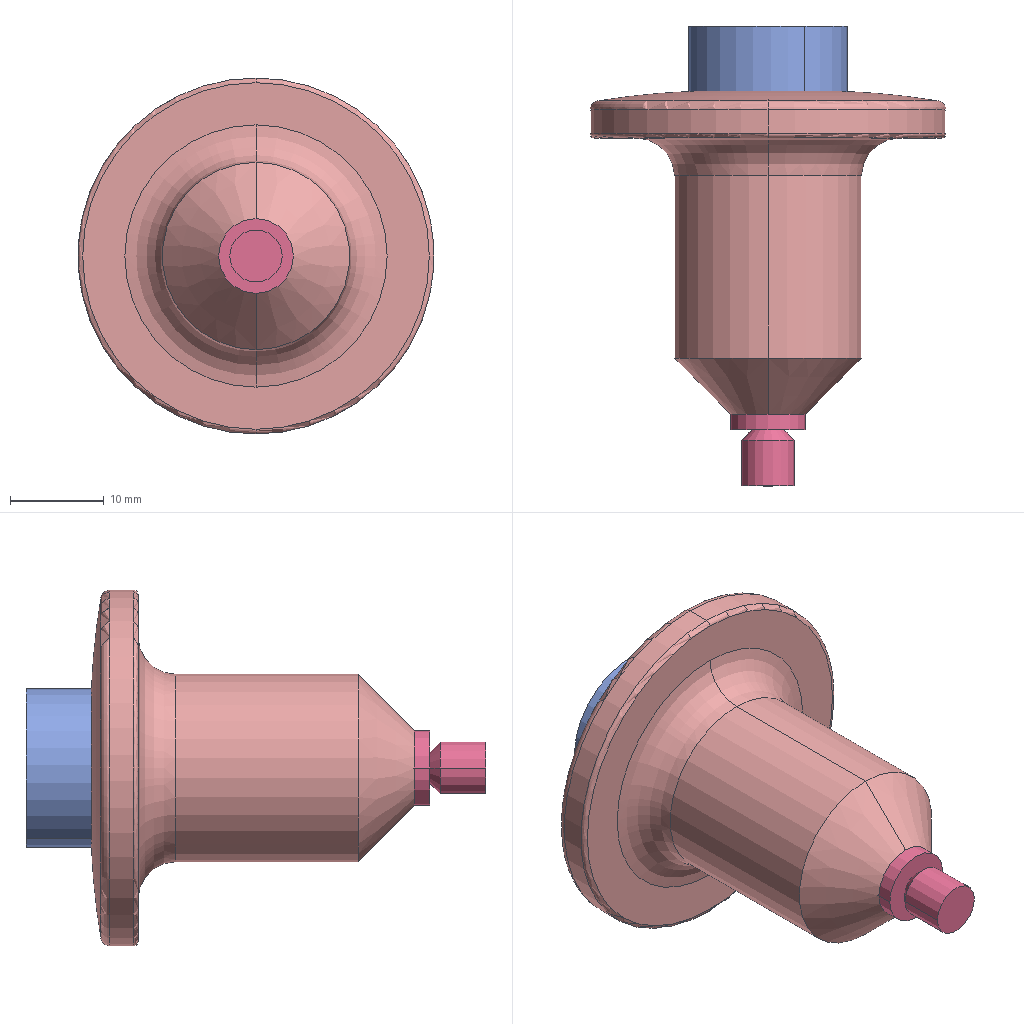Assembly | SolidWorks | 7 different items | 7 placed | box 38 x 49 x 38 mm
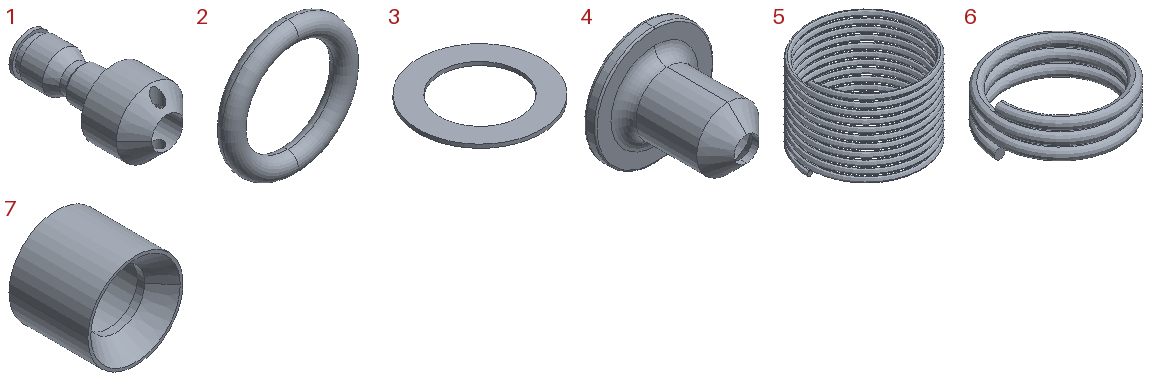Parts list (item | quantity | size | volume | features):
1 | x1 | 17 x 35.31 x 17 mm | 3384 mm3 | features Cut 1, ICE 1, MirrorPattern 1, RevCut 1, Revolution 1
2 | x1 | 12.043 x 1.84 x 12.043 mm | 85.235 mm3 | features Sweep 1
3 | x1 | 17 x 17 x 0.5 mm | 65.973 mm3 | features Extrusion 1
4 | x1 | 38 x 34.477 x 38 mm | 6932 mm3 | features Cut 1, ICE 1, Revolution 1
5 | x1 | 5.75 x 5.75 x 4.25 mm | 9.284 mm3 | features Helix 1, Sweep 1
6 | x1 | 17 x 17 x 6.999 mm | 258.247 mm3 | features Helix 1, Sweep 1
7 | x1 | 17 x 14.11 x 17 mm | 1515 mm3 | features Revolution 1
Mates (type | each side: item.copy, entity, surface, feature):
Concentric | 4.1 face cylinder Revolve1 | 7.1 face cylinder Revolve1
Concentric | 4.1 face cylinder Revolve1 | 1.1 face cylinder Revolve1
Concentric | 4.1 face cylinder Revolve1 | 6.1 select_type:24
Concentric | 1.1 edge | 5.1 select_type:24
Coincident | 1.1 face plane Cut-Extrude2 | 5.1 select_type:24
Concentric | 4.1 face cylinder Revolve1 | 3.1 face cylinder Boss-Extrude1
Coincident | 1.1 face plane Revolve1 | 6.1 select_type:24
Coincident | 4.1 edge | 3.1 face plane Boss-Extrude1
Concentric | 1.1 face cylinder Revolve1 | 2.1 select_type:24
Coincident | 1.1 face plane Revolve1 | 2.1 select_type:24
LimitDistanceDim | 1.1 face plane Revolve1 | 7.1 face plane Revolve1
Coincident | 1.1 axis | assembly plane